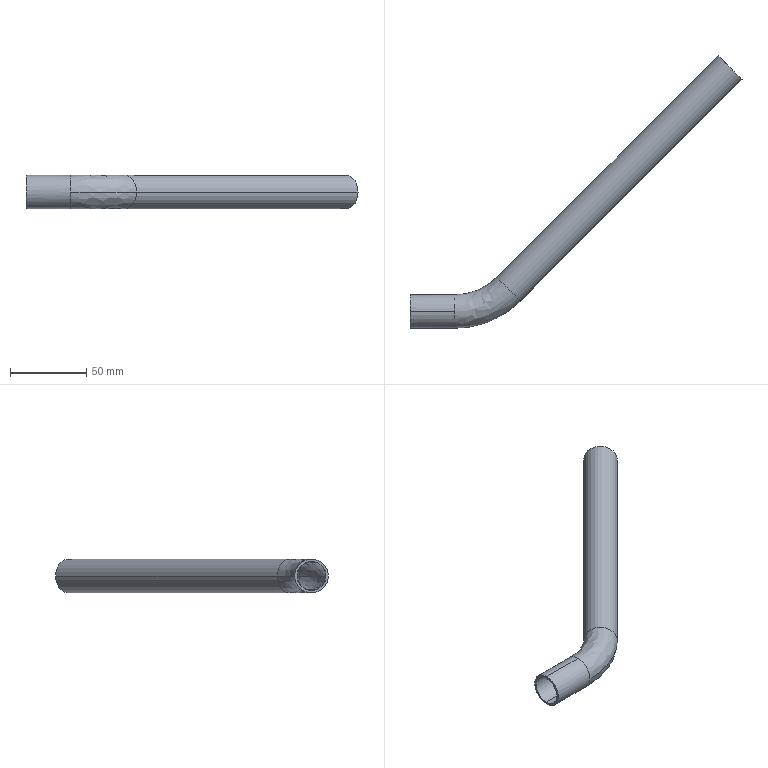Part | STEP file | copper tube 7_default_machined_ | 1 solid | 14 faces | box 217.778 x 178.778 x 22 mm | volume 26481 mm3 | cylinder 8 | spline 4 | plane 2 | commonest cylinder face diameters 19 x4 22 x4